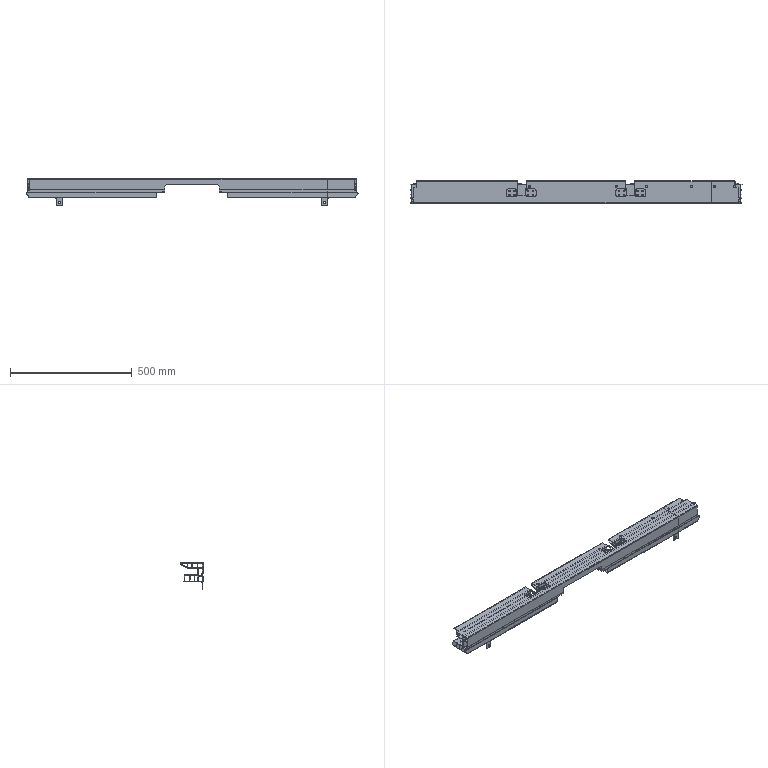Part | 2 solids | 901 faces | box 1365 x 90.95 x 108.501 mm | volume 1740958 mm3 | cylinder 533 | plane 355 | cone 7 | spline 6 | commonest cylinder face diameters 4 x171 7 x96 9 x48 1 x43 2 x42 17 x36